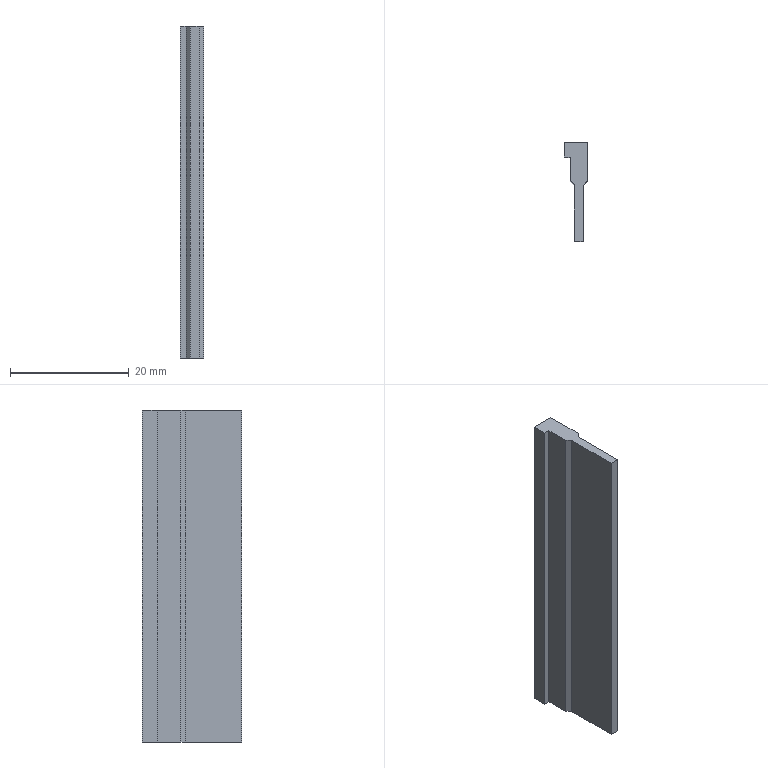Part | NX | features BREP 2 | 2 solids | 24 faces | box 3.95 x 16.702 x 56 mm | volume 4199 mm3 | plane 24
STEP:
#1=CARTESIAN_POINT('',(1.225,-8.351,-4.));
#2=VERTEX_POINT('',#1);
#3=CARTESIAN_POINT('',(1.225,-8.351,52.));
#4=VERTEX_POINT('',#3);
#5=CARTESIAN_POINT('',(1.225,-8.351,0.));
#6=DIRECTION('',(0.,0.,1.));
#7=VECTOR('',#6,1000.);
#8=LINE('',#5,#7);
#9=EDGE_CURVE('',#2,#4,#8,.T.);
#10=ORIENTED_EDGE('',*,*,#9,.F.);
#11=CARTESIAN_POINT('',(1.225,1.11,-4.));
#12=VERTEX_POINT('',#11);
#13=CARTESIAN_POINT('',(1.225,-22.649,-4.));
#14=DIRECTION('',(0.,1.,0.));
#15=VECTOR('',#14,1000.);
#16=LINE('',#13,#15);
#17=EDGE_CURVE('',#2,#12,#16,.T.);
#18=ORIENTED_EDGE('',*,*,#17,.T.);
#19=CARTESIAN_POINT('',(1.225,1.11,52.));
#20=VERTEX_POINT('',#19);
#21=CARTESIAN_POINT('',(1.225,1.11,0.));
#22=DIRECTION('',(0.,0.,1.));
#23=VECTOR('',#22,1000.);
#24=LINE('',#21,#23);
#25=EDGE_CURVE('',#12,#20,#24,.T.);
#26=ORIENTED_EDGE('',*,*,#25,.T.);
#27=CARTESIAN_POINT('',(1.225,-22.649,52.));
#28=DIRECTION('',(0.,1.,0.));
#29=VECTOR('',#28,1000.);
#30=LINE('',#27,#29);
#31=EDGE_CURVE('',#4,#20,#30,.T.);
#32=ORIENTED_EDGE('',*,*,#31,.F.);
#33=EDGE_LOOP('',(#10,#18,#26,#32));
#34=FACE_BOUND('',#33,.T.);
#35=CARTESIAN_POINT('',(1.225,-5.351,0.));
#36=DIRECTION('',(-1.,0.,0.));
#37=DIRECTION('',(0.,1.,0.));
#38=AXIS2_PLACEMENT_3D('',#35,#36,#37);
#39=PLANE('',#38);
#40=ADVANCED_FACE('',(#34),#39,.F.);
#41=ORIENTED_EDGE('',*,*,#9,.T.);
#42=CARTESIAN_POINT('',(-0.275,-8.351,52.));
#43=VERTEX_POINT('',#42);
#44=CARTESIAN_POINT('',(0.683,-8.351,52.));
#45=DIRECTION('',(1.,0.,0.));
#46=VECTOR('',#45,1000.);
#47=LINE('',#44,#46);
#48=EDGE_CURVE('',#43,#4,#47,.T.);
#49=ORIENTED_EDGE('',*,*,#48,.F.);
#50=CARTESIAN_POINT('',(-0.275,-8.351,-4.));
#51=VERTEX_POINT('',#50);
#52=CARTESIAN_POINT('',(-0.275,-8.351,0.));
#53=DIRECTION('',(0.,0.,1.));
#54=VECTOR('',#53,1000.);
#55=LINE('',#52,#54);
#56=EDGE_CURVE('',#51,#43,#55,.T.);
#57=ORIENTED_EDGE('',*,*,#56,.F.);
#58=CARTESIAN_POINT('',(0.683,-8.351,-4.));
#59=DIRECTION('',(1.,0.,0.));
#60=VECTOR('',#59,1000.);
#61=LINE('',#58,#60);
#62=EDGE_CURVE('',#51,#2,#61,.T.);
#63=ORIENTED_EDGE('',*,*,#62,.T.);
#64=EDGE_LOOP('',(#41,#49,#57,#63));
#65=FACE_BOUND('',#64,.T.);
#66=CARTESIAN_POINT('',(0.683,-8.351,0.));
#67=DIRECTION('',(0.,-1.,0.));
#68=DIRECTION('',(-1.,0.,0.));
#69=AXIS2_PLACEMENT_3D('',#66,#67,#68);
#70=PLANE('',#69);
#71=ADVANCED_FACE('',(#65),#70,.T.);
#72=CARTESIAN_POINT('',(-0.275,1.16,-4.));
#73=VERTEX_POINT('',#72);
#74=CARTESIAN_POINT('',(-0.275,1.16,52.));
#75=VERTEX_POINT('',#74);
#76=CARTESIAN_POINT('',(-0.275,1.16,0.));
#77=DIRECTION('',(0.,0.,1.));
#78=VECTOR('',#77,1000.);
#79=LINE('',#76,#78);
#80=EDGE_CURVE('',#73,#75,#79,.T.);
#81=ORIENTED_EDGE('',*,*,#80,.F.);
#82=CARTESIAN_POINT('',(-0.275,-22.649,-4.));
#83=DIRECTION('',(0.,-1.,0.));
#84=VECTOR('',#83,1000.);
#85=LINE('',#82,#84);
#86=EDGE_CURVE('',#73,#51,#85,.T.);
#87=ORIENTED_EDGE('',*,*,#86,.T.);
#88=ORIENTED_EDGE('',*,*,#56,.T.);
#89=CARTESIAN_POINT('',(-0.275,-22.649,52.));
#90=DIRECTION('',(0.,-1.,0.));
#91=VECTOR('',#90,1000.);
#92=LINE('',#89,#91);
#93=EDGE_CURVE('',#75,#43,#92,.T.);
#94=ORIENTED_EDGE('',*,*,#93,.F.);
#95=EDGE_LOOP('',(#81,#87,#88,#94));
#96=FACE_BOUND('',#95,.T.);
#97=CARTESIAN_POINT('',(-0.275,-4.148,0.));
#98=DIRECTION('',(1.,0.,0.));
#99=DIRECTION('',(0.,-1.,0.));
#100=AXIS2_PLACEMENT_3D('',#97,#98,#99);
#101=PLANE('',#100);
#102=ADVANCED_FACE('',(#96),#101,.F.);
#103=ORIENTED_EDGE('',*,*,#80,.T.);
#104=CARTESIAN_POINT('',(-0.975,1.86,52.));
#105=VERTEX_POINT('',#104);
#106=CARTESIAN_POINT('',(-0.275,1.16,52.));
#107=DIRECTION('',(0.7071,-0.7071,0.));
#108=VECTOR('',#107,1000.);
#109=LINE('',#106,#108);
#110=EDGE_CURVE('',#105,#75,#109,.T.);
#111=ORIENTED_EDGE('',*,*,#110,.F.);
#112=CARTESIAN_POINT('',(-0.975,1.86,-4.));
#113=VERTEX_POINT('',#112);
#114=CARTESIAN_POINT('',(-0.975,1.86,0.));
#115=DIRECTION('',(0.,0.,1.));
#116=VECTOR('',#115,1000.);
#117=LINE('',#114,#116);
#118=EDGE_CURVE('',#113,#105,#117,.T.);
#119=ORIENTED_EDGE('',*,*,#118,.F.);
#120=CARTESIAN_POINT('',(-0.275,1.16,-4.));
#121=DIRECTION('',(0.7071,-0.7071,0.));
#122=VECTOR('',#121,1000.);
#123=LINE('',#120,#122);
#124=EDGE_CURVE('',#113,#73,#123,.T.);
#125=ORIENTED_EDGE('',*,*,#124,.T.);
#126=EDGE_LOOP('',(#103,#111,#119,#125));
#127=FACE_BOUND('',#126,.T.);
#128=CARTESIAN_POINT('',(-0.275,1.16,0.));
#129=DIRECTION('',(0.7071,0.7071,0.));
#130=DIRECTION('',(0.7071,-0.7071,0.));
#131=AXIS2_PLACEMENT_3D('',#128,#129,#130);
#132=PLANE('',#131);
#133=ADVANCED_FACE('',(#127),#132,.F.);
#134=ORIENTED_EDGE('',*,*,#118,.T.);
#135=CARTESIAN_POINT('',(-0.975,5.852,52.));
#136=VERTEX_POINT('',#135);
#137=CARTESIAN_POINT('',(-0.975,-22.649,52.));
#138=DIRECTION('',(0.,-1.,0.));
#139=VECTOR('',#138,1000.);
#140=LINE('',#137,#139);
#141=EDGE_CURVE('',#136,#105,#140,.T.);
#142=ORIENTED_EDGE('',*,*,#141,.F.);
#143=CARTESIAN_POINT('',(-0.975,5.852,-4.));
#144=VERTEX_POINT('',#143);
#145=CARTESIAN_POINT('',(-0.975,5.852,0.));
#146=DIRECTION('',(0.,0.,1.));
#147=VECTOR('',#146,1000.);
#148=LINE('',#145,#147);
#149=EDGE_CURVE('',#144,#136,#148,.T.);
#150=ORIENTED_EDGE('',*,*,#149,.F.);
#151=CARTESIAN_POINT('',(-0.975,-22.649,-4.));
#152=DIRECTION('',(0.,-1.,0.));
#153=VECTOR('',#152,1000.);
#154=LINE('',#151,#153);
#155=EDGE_CURVE('',#144,#113,#154,.T.);
#156=ORIENTED_EDGE('',*,*,#155,.T.);
#157=EDGE_LOOP('',(#134,#142,#150,#156));
#158=FACE_BOUND('',#157,.T.);
#159=CARTESIAN_POINT('',(-0.975,1.86,0.));
#160=DIRECTION('',(1.,0.,0.));
#161=DIRECTION('',(0.,-1.,0.));
#162=AXIS2_PLACEMENT_3D('',#159,#160,#161);
#163=PLANE('',#162);
#164=ADVANCED_FACE('',(#158),#163,.F.);
#165=ORIENTED_EDGE('',*,*,#149,.T.);
#166=CARTESIAN_POINT('',(-1.975,5.852,52.));
#167=VERTEX_POINT('',#166);
#168=CARTESIAN_POINT('',(0.683,5.852,52.));
#169=DIRECTION('',(1.,0.,0.));
#170=VECTOR('',#169,1000.);
#171=LINE('',#168,#170);
#172=EDGE_CURVE('',#167,#136,#171,.T.);
#173=ORIENTED_EDGE('',*,*,#172,.F.);
#174=CARTESIAN_POINT('',(-1.975,5.852,-4.));
#175=VERTEX_POINT('',#174);
#176=CARTESIAN_POINT('',(-1.975,5.852,0.));
#177=DIRECTION('',(0.,0.,1.));
#178=VECTOR('',#177,1000.);
#179=LINE('',#176,#178);
#180=EDGE_CURVE('',#175,#167,#179,.T.);
#181=ORIENTED_EDGE('',*,*,#180,.F.);
#182=CARTESIAN_POINT('',(0.683,5.852,-4.));
#183=DIRECTION('',(1.,0.,0.));
#184=VECTOR('',#183,1000.);
#185=LINE('',#182,#184);
#186=EDGE_CURVE('',#175,#144,#185,.T.);
#187=ORIENTED_EDGE('',*,*,#186,.T.);
#188=EDGE_LOOP('',(#165,#173,#181,#187));
#189=FACE_BOUND('',#188,.T.);
#190=CARTESIAN_POINT('',(-0.975,5.852,0.));
#191=DIRECTION('',(0.,1.,0.));
#192=DIRECTION('',(1.,0.,0.));
#193=AXIS2_PLACEMENT_3D('',#190,#191,#192);
#194=PLANE('',#193);
#195=ADVANCED_FACE('',(#189),#194,.F.);
#196=ORIENTED_EDGE('',*,*,#180,.T.);
#197=CARTESIAN_POINT('',(-1.975,8.351,52.));
#198=VERTEX_POINT('',#197);
#199=CARTESIAN_POINT('',(-1.975,-22.649,52.));
#200=DIRECTION('',(0.,-1.,0.));
#201=VECTOR('',#200,1000.);
#202=LINE('',#199,#201);
#203=EDGE_CURVE('',#198,#167,#202,.T.);
#204=ORIENTED_EDGE('',*,*,#203,.F.);
#205=CARTESIAN_POINT('',(-1.975,8.351,-4.));
#206=VERTEX_POINT('',#205);
#207=CARTESIAN_POINT('',(-1.975,8.351,0.));
#208=DIRECTION('',(0.,0.,1.));
#209=VECTOR('',#208,1000.);
#210=LINE('',#207,#209);
#211=EDGE_CURVE('',#206,#198,#210,.T.);
#212=ORIENTED_EDGE('',*,*,#211,.F.);
#213=CARTESIAN_POINT('',(-1.975,-22.649,-4.));
#214=DIRECTION('',(0.,-1.,0.));
#215=VECTOR('',#214,1000.);
#216=LINE('',#213,#215);
#217=EDGE_CURVE('',#206,#175,#216,.T.);
#218=ORIENTED_EDGE('',*,*,#217,.T.);
#219=EDGE_LOOP('',(#196,#204,#212,#218));
#220=FACE_BOUND('',#219,.T.);
#221=CARTESIAN_POINT('',(-1.975,-22.649,0.));
#222=DIRECTION('',(1.,0.,0.));
#223=DIRECTION('',(0.,-1.,0.));
#224=AXIS2_PLACEMENT_3D('',#221,#222,#223);
#225=PLANE('',#224);
#226=ADVANCED_FACE('',(#220),#225,.F.);
#227=ORIENTED_EDGE('',*,*,#211,.T.);
#228=CARTESIAN_POINT('',(1.975,8.351,52.));
#229=VERTEX_POINT('',#228);
#230=CARTESIAN_POINT('',(0.683,8.351,52.));
#231=DIRECTION('',(-1.,0.,0.));
#232=VECTOR('',#231,1000.);
#233=LINE('',#230,#232);
#234=EDGE_CURVE('',#229,#198,#233,.T.);
#235=ORIENTED_EDGE('',*,*,#234,.F.);
#236=CARTESIAN_POINT('',(1.975,8.351,-4.));
#237=VERTEX_POINT('',#236);
#238=CARTESIAN_POINT('',(1.975,8.351,0.));
#239=DIRECTION('',(0.,0.,1.));
#240=VECTOR('',#239,1000.);
#241=LINE('',#238,#240);
#242=EDGE_CURVE('',#237,#229,#241,.T.);
#243=ORIENTED_EDGE('',*,*,#242,.F.);
#244=CARTESIAN_POINT('',(0.683,8.351,-4.));
#245=DIRECTION('',(-1.,0.,0.));
#246=VECTOR('',#245,1000.);
#247=LINE('',#244,#246);
#248=EDGE_CURVE('',#237,#206,#247,.T.);
#249=ORIENTED_EDGE('',*,*,#248,.T.);
#250=EDGE_LOOP('',(#227,#235,#243,#249));
#251=FACE_BOUND('',#250,.T.);
#252=CARTESIAN_POINT('',(-21.567,8.351,0.));
#253=DIRECTION('',(0.,-1.,0.));
#254=DIRECTION('',(-1.,0.,0.));
#255=AXIS2_PLACEMENT_3D('',#252,#253,#254);
#256=PLANE('',#255);
#257=ADVANCED_FACE('',(#251),#256,.F.);
#258=ORIENTED_EDGE('',*,*,#242,.T.);
#259=CARTESIAN_POINT('',(1.975,1.86,52.));
#260=VERTEX_POINT('',#259);
#261=CARTESIAN_POINT('',(1.975,-22.649,52.));
#262=DIRECTION('',(0.,1.,0.));
#263=VECTOR('',#262,1000.);
#264=LINE('',#261,#263);
#265=EDGE_CURVE('',#260,#229,#264,.T.);
#266=ORIENTED_EDGE('',*,*,#265,.F.);
#267=CARTESIAN_POINT('',(1.975,1.86,-4.));
#268=VERTEX_POINT('',#267);
#269=CARTESIAN_POINT('',(1.975,1.86,0.));
#270=DIRECTION('',(0.,0.,1.));
#271=VECTOR('',#270,1000.);
#272=LINE('',#269,#271);
#273=EDGE_CURVE('',#268,#260,#272,.T.);
#274=ORIENTED_EDGE('',*,*,#273,.F.);
#275=CARTESIAN_POINT('',(1.975,-22.649,-4.));
#276=DIRECTION('',(0.,1.,0.));
#277=VECTOR('',#276,1000.);
#278=LINE('',#275,#277);
#279=EDGE_CURVE('',#268,#237,#278,.T.);
#280=ORIENTED_EDGE('',*,*,#279,.T.);
#281=EDGE_LOOP('',(#258,#266,#274,#280));
#282=FACE_BOUND('',#281,.T.);
#283=CARTESIAN_POINT('',(1.975,5.852,0.));
#284=DIRECTION('',(-1.,0.,0.));
#285=DIRECTION('',(0.,1.,0.));
#286=AXIS2_PLACEMENT_3D('',#283,#284,#285);
#287=PLANE('',#286);
#288=ADVANCED_FACE('',(#282),#287,.F.);
#289=CARTESIAN_POINT('',(1.975,1.86,-4.));
#290=DIRECTION('',(0.7071,0.7071,0.));
#291=VECTOR('',#290,1000.);
#292=LINE('',#289,#291);
#293=EDGE_CURVE('',#12,#268,#292,.T.);
#294=ORIENTED_EDGE('',*,*,#293,.T.);
#295=ORIENTED_EDGE('',*,*,#273,.T.);
#296=CARTESIAN_POINT('',(1.975,1.86,52.));
#297=DIRECTION('',(0.7071,0.7071,0.));
#298=VECTOR('',#297,1000.);
#299=LINE('',#296,#298);
#300=EDGE_CURVE('',#20,#260,#299,.T.);
#301=ORIENTED_EDGE('',*,*,#300,.F.);
#302=ORIENTED_EDGE('',*,*,#25,.F.);
#303=EDGE_LOOP('',(#294,#295,#301,#302));
#304=FACE_BOUND('',#303,.T.);
#305=CARTESIAN_POINT('',(1.975,1.86,0.));
#306=DIRECTION('',(-0.7071,0.7071,0.));
#307=DIRECTION('',(0.7071,0.7071,0.));
#308=AXIS2_PLACEMENT_3D('',#305,#306,#307);
#309=PLANE('',#308);
#310=ADVANCED_FACE('',(#304),#309,.F.);
#311=ORIENTED_EDGE('',*,*,#265,.T.);
#312=ORIENTED_EDGE('',*,*,#234,.T.);
#313=ORIENTED_EDGE('',*,*,#203,.T.);
#314=ORIENTED_EDGE('',*,*,#172,.T.);
#315=ORIENTED_EDGE('',*,*,#141,.T.);
#316=ORIENTED_EDGE('',*,*,#110,.T.);
#317=ORIENTED_EDGE('',*,*,#93,.T.);
#318=ORIENTED_EDGE('',*,*,#48,.T.);
#319=ORIENTED_EDGE('',*,*,#31,.T.);
#320=ORIENTED_EDGE('',*,*,#300,.T.);
#321=EDGE_LOOP('',(#311,#312,#313,#314,#315,#316,#317,#318,#319,#320));
#322=FACE_BOUND('',#321,.T.);
#323=CARTESIAN_POINT('',(0.683,-22.649,52.));
#324=DIRECTION('',(0.,0.,1.));
#325=DIRECTION('',(-1.,0.,0.));
#326=AXIS2_PLACEMENT_3D('',#323,#324,#325);
#327=PLANE('',#326);
#328=ADVANCED_FACE('',(#322),#327,.T.);
#329=ORIENTED_EDGE('',*,*,#279,.F.);
#330=ORIENTED_EDGE('',*,*,#293,.F.);
#331=ORIENTED_EDGE('',*,*,#17,.F.);
#332=ORIENTED_EDGE('',*,*,#62,.F.);
#333=ORIENTED_EDGE('',*,*,#86,.F.);
#334=ORIENTED_EDGE('',*,*,#124,.F.);
#335=ORIENTED_EDGE('',*,*,#155,.F.);
#336=ORIENTED_EDGE('',*,*,#186,.F.);
#337=ORIENTED_EDGE('',*,*,#217,.F.);
#338=ORIENTED_EDGE('',*,*,#248,.F.);
#339=EDGE_LOOP('',(#329,#330,#331,#332,#333,#334,#335,#336,#337,#338));
#340=FACE_BOUND('',#339,.T.);
#341=CARTESIAN_POINT('',(0.683,-22.649,-4.));
#342=DIRECTION('',(0.,0.,1.));
#343=DIRECTION('',(-1.,0.,0.));
#344=AXIS2_PLACEMENT_3D('',#341,#342,#343);
#345=PLANE('',#344);
#346=ADVANCED_FACE('',(#340),#345,.F.);
#347=CLOSED_SHELL('',(#40,#71,#102,#133,#164,#195,#226,#257,#288,#310,#328,#346));
#348=MANIFOLD_SOLID_BREP('',#347);
#349=CARTESIAN_POINT('',(1.225,-8.351,-4.));
#350=VERTEX_POINT('',#349);
#351=CARTESIAN_POINT('',(1.225,-8.351,52.));
#352=VERTEX_POINT('',#351);
#353=CARTESIAN_POINT('',(1.225,-8.351,0.));
#354=DIRECTION('',(0.,0.,1.));
#355=VECTOR('',#354,1000.);
#356=LINE('',#353,#355);
#357=EDGE_CURVE('',#350,#352,#356,.T.);
#358=ORIENTED_EDGE('',*,*,#357,.F.);
#359=CARTESIAN_POINT('',(1.225,1.11,-4.));
#360=VERTEX_POINT('',#359);
#361=CARTESIAN_POINT('',(1.225,-22.649,-4.));
#362=DIRECTION('',(0.,1.,0.));
#363=VECTOR('',#362,1000.);
#364=LINE('',#361,#363);
#365=EDGE_CURVE('',#350,#360,#364,.T.);
#366=ORIENTED_EDGE('',*,*,#365,.T.);
#367=CARTESIAN_POINT('',(1.225,1.11,52.));
#368=VERTEX_POINT('',#367);
#369=CARTESIAN_POINT('',(1.225,1.11,0.));
#370=DIRECTION('',(0.,0.,1.));
#371=VECTOR('',#370,1000.);
#372=LINE('',#369,#371);
#373=EDGE_CURVE('',#360,#368,#372,.T.);
#374=ORIENTED_EDGE('',*,*,#373,.T.);
#375=CARTESIAN_POINT('',(1.225,-22.649,52.));
#376=DIRECTION('',(0.,1.,0.));
#377=VECTOR('',#376,1000.);
#378=LINE('',#375,#377);
#379=EDGE_CURVE('',#352,#368,#378,.T.);
#380=ORIENTED_EDGE('',*,*,#379,.F.);
#381=EDGE_LOOP('',(#358,#366,#374,#380));
#382=FACE_BOUND('',#381,.T.);
#383=CARTESIAN_POINT('',(1.225,-5.351,0.));
#384=DIRECTION('',(-1.,0.,0.));
#385=DIRECTION('',(0.,1.,0.));
#386=AXIS2_PLACEMENT_3D('',#383,#384,#385);
#387=PLANE('',#386);
#388=ADVANCED_FACE('',(#382),#387,.F.);
#389=ORIENTED_EDGE('',*,*,#357,.T.);
#390=CARTESIAN_POINT('',(-0.275,-8.351,52.));
#391=VERTEX_POINT('',#390);
#392=CARTESIAN_POINT('',(0.683,-8.351,52.));
#393=DIRECTION('',(1.,0.,0.));
#394=VECTOR('',#393,1000.);
#395=LINE('',#392,#394);
#396=EDGE_CURVE('',#391,#352,#395,.T.);
#397=ORIENTED_EDGE('',*,*,#396,.F.);
#398=CARTESIAN_POINT('',(-0.275,-8.351,-4.));
#399=VERTEX_POINT('',#398);
#400=CARTESIAN_POINT('',(-0.275,-8.351,0.));
#401=DIRECTION('',(0.,0.,1.));
#402=VECTOR('',#401,1000.);
#403=LINE('',#400,#402);
#404=EDGE_CURVE('',#399,#391,#403,.T.);
#405=ORIENTED_EDGE('',*,*,#404,.F.);
#406=CARTESIAN_POINT('',(0.683,-8.351,-4.));
#407=DIRECTION('',(1.,0.,0.));
#408=VECTOR('',#407,1000.);
#409=LINE('',#406,#408);
#410=EDGE_CURVE('',#399,#350,#409,.T.);
#411=ORIENTED_EDGE('',*,*,#410,.T.);
#412=EDGE_LOOP('',(#389,#397,#405,#411));
#413=FACE_BOUND('',#412,.T.);
#414=CARTESIAN_POINT('',(0.683,-8.351,0.));
#415=DIRECTION('',(0.,-1.,0.));
#416=DIRECTION('',(-1.,0.,0.));
#417=AXIS2_PLACEMENT_3D('',#414,#415,#416);
#418=PLANE('',#417);
#419=ADVANCED_FACE('',(#413),#418,.T.);
#420=CARTESIAN_POINT('',(-0.275,1.16,-4.));
#421=VERTEX_POINT('',#420);
#422=CARTESIAN_POINT('',(-0.275,1.16,52.));
#423=VERTEX_POINT('',#422);
#424=CARTESIAN_POINT('',(-0.275,1.16,0.));
#425=DIRECTION('',(0.,0.,1.));
#426=VECTOR('',#425,1000.);
#427=LINE('',#424,#426);
#428=EDGE_CURVE('',#421,#423,#427,.T.);
#429=ORIENTED_EDGE('',*,*,#428,.F.);
#430=CARTESIAN_POINT('',(-0.275,-22.649,-4.));
#431=DIRECTION('',(0.,-1.,0.));
#432=VECTOR('',#431,1000.);
#433=LINE('',#430,#432);
#434=EDGE_CURVE('',#421,#399,#433,.T.);
#435=ORIENTED_EDGE('',*,*,#434,.T.);
#436=ORIENTED_EDGE('',*,*,#404,.T.);
#437=CARTESIAN_POINT('',(-0.275,-22.649,52.));
#438=DIRECTION('',(0.,-1.,0.));
#439=VECTOR('',#438,1000.);
#440=LINE('',#437,#439);
#441=EDGE_CURVE('',#423,#391,#440,.T.);
#442=ORIENTED_EDGE('',*,*,#441,.F.);
#443=EDGE_LOOP('',(#429,#435,#436,#442));
#444=FACE_BOUND('',#443,.T.);
#445=CARTESIAN_POINT('',(-0.275,-4.148,0.));
#446=DIRECTION('',(1.,0.,0.));
#447=DIRECTION('',(0.,-1.,0.));
#448=AXIS2_PLACEMENT_3D('',#445,#446,#447);
#449=PLANE('',#448);
#450=ADVANCED_FACE('',(#444),#449,.F.);
#451=ORIENTED_EDGE('',*,*,#428,.T.);
#452=CARTESIAN_POINT('',(-0.975,1.86,52.));
#453=VERTEX_POINT('',#452);
#454=CARTESIAN_POINT('',(-0.275,1.16,52.));
#455=DIRECTION('',(0.7071,-0.7071,0.));
#456=VECTOR('',#455,1000.);
#457=LINE('',#454,#456);
#458=EDGE_CURVE('',#453,#423,#457,.T.);
#459=ORIENTED_EDGE('',*,*,#458,.F.);
#460=CARTESIAN_POINT('',(-0.975,1.86,-4.));
#461=VERTEX_POINT('',#460);
#462=CARTESIAN_POINT('',(-0.975,1.86,0.));
#463=DIRECTION('',(0.,0.,1.));
#464=VECTOR('',#463,1000.);
#465=LINE('',#462,#464);
#466=EDGE_CURVE('',#461,#453,#465,.T.);
#467=ORIENTED_EDGE('',*,*,#466,.F.);
#468=CARTESIAN_POINT('',(-0.275,1.16,-4.));
#469=DIRECTION('',(0.7071,-0.7071,0.));
#470=VECTOR('',#469,1000.);
#471=LINE('',#468,#470);
#472=EDGE_CURVE('',#461,#421,#471,.T.);
#473=ORIENTED_EDGE('',*,*,#472,.T.);
#474=EDGE_LOOP('',(#451,#459,#467,#473));
#475=FACE_BOUND('',#474,.T.);
#476=CARTESIAN_POINT('',(-0.275,1.16,0.));
#477=DIRECTION('',(0.7071,0.7071,0.));
#478=DIRECTION('',(0.7071,-0.7071,0.));
#479=AXIS2_PLACEMENT_3D('',#476,#477,#478);
#480=PLANE('',#479);
#481=ADVANCED_FACE('',(#475),#480,.F.);
#482=ORIENTED_EDGE('',*,*,#466,.T.);
#483=CARTESIAN_POINT('',(-0.975,5.852,52.));
#484=VERTEX_POINT('',#483);
#485=CARTESIAN_POINT('',(-0.975,-22.649,52.));
#486=DIRECTION('',(0.,-1.,0.));
#487=VECTOR('',#486,1000.);
#488=LINE('',#485,#487);
#489=EDGE_CURVE('',#484,#453,#488,.T.);
#490=ORIENTED_EDGE('',*,*,#489,.F.);
#491=CARTESIAN_POINT('',(-0.975,5.852,-4.));
#492=VERTEX_POINT('',#491);
#493=CARTESIAN_POINT('',(-0.975,5.852,0.));
#494=DIRECTION('',(0.,0.,1.));
#495=VECTOR('',#494,1000.);
#496=LINE('',#493,#495);
#497=EDGE_CURVE('',#492,#484,#496,.T.);
#498=ORIENTED_EDGE('',*,*,#497,.F.);
#499=CARTESIAN_POINT('',(-0.975,-22.649,-4.));
#500=DIRECTION('',(0.,-1.,0.));
#501=VECTOR('',#500,1000.);
#502=LINE('',#499,#501);
#503=EDGE_CURVE('',#492,#461,#502,.T.);
#504=ORIENTED_EDGE('',*,*,#503,.T.);
#505=EDGE_LOOP('',(#482,#490,#498,#504));
#506=FACE_BOUND('',#505,.T.);
#507=CARTESIAN_POINT('',(-0.975,1.86,0.));
#508=DIRECTION('',(1.,0.,0.));
#509=DIRECTION('',(0.,-1.,0.));
#510=AXIS2_PLACEMENT_3D('',#507,#508,#509);
#511=PLANE('',#510);
#512=ADVANCED_FACE('',(#506),#511,.F.);
#513=ORIENTED_EDGE('',*,*,#497,.T.);
#514=CARTESIAN_POINT('',(-1.975,5.852,52.));
#515=VERTEX_POINT('',#514);
#516=CARTESIAN_POINT('',(0.683,5.852,52.));
#517=DIRECTION('',(1.,0.,0.));
#518=VECTOR('',#517,1000.);
#519=LINE('',#516,#518);
#520=EDGE_CURVE('',#515,#484,#519,.T.);
#521=ORIENTED_EDGE('',*,*,#520,.F.);
#522=CARTESIAN_POINT('',(-1.975,5.852,-4.));
#523=VERTEX_POINT('',#522);
#524=CARTESIAN_POINT('',(-1.975,5.852,0.));
#525=DIRECTION('',(0.,0.,1.));
#526=VECTOR('',#525,1000.);
#527=LINE('',#524,#526);
#528=EDGE_CURVE('',#523,#515,#527,.T.);
#529=ORIENTED_EDGE('',*,*,#528,.F.);
#530=CARTESIAN_POINT('',(0.683,5.852,-4.));
#531=DIRECTION('',(1.,0.,0.));
#532=VECTOR('',#531,1000.);
#533=LINE('',#530,#532);
#534=EDGE_CURVE('',#523,#492,#533,.T.);
#535=ORIENTED_EDGE('',*,*,#534,.T.);
#536=EDGE_LOOP('',(#513,#521,#529,#535));
#537=FACE_BOUND('',#536,.T.);
#538=CARTESIAN_POINT('',(-0.975,5.852,0.));
#539=DIRECTION('',(0.,1.,0.));
#540=DIRECTION('',(1.,0.,0.));
#541=AXIS2_PLACEMENT_3D('',#538,#539,#540);
#542=PLANE('',#541);
#543=ADVANCED_FACE('',(#537),#542,.F.);
#544=ORIENTED_EDGE('',*,*,#528,.T.);
#545=CARTESIAN_POINT('',(-1.975,8.351,52.));
#546=VERTEX_POINT('',#545);
#547=CARTESIAN_POINT('',(-1.975,-22.649,52.));
#548=DIRECTION('',(0.,-1.,0.));
#549=VECTOR('',#548,1000.);
#550=LINE('',#547,#549);
#551=EDGE_CURVE('',#546,#515,#550,.T.);
#552=ORIENTED_EDGE('',*,*,#551,.F.);
#553=CARTESIAN_POINT('',(-1.975,8.351,-4.));
#554=VERTEX_POINT('',#553);
#555=CARTESIAN_POINT('',(-1.975,8.351,0.));
#556=DIRECTION('',(0.,0.,1.));
#557=VECTOR('',#556,1000.);
#558=LINE('',#555,#557);
#559=EDGE_CURVE('',#554,#546,#558,.T.);
#560=ORIENTED_EDGE('',*,*,#559,.F.);
#561=CARTESIAN_POINT('',(-1.975,-22.649,-4.));
#562=DIRECTION('',(0.,-1.,0.));
#563=VECTOR('',#562,1000.);
#564=LINE('',#561,#563);
#565=EDGE_CURVE('',#554,#523,#564,.T.);
#566=ORIENTED_EDGE('',*,*,#565,.T.);
#567=EDGE_LOOP('',(#544,#552,#560,#566));
#568=FACE_BOUND('',#567,.T.);
#569=CARTESIAN_POINT('',(-1.975,-22.649,0.));
#570=DIRECTION('',(1.,0.,0.));
#571=DIRECTION('',(0.,-1.,0.));
#572=AXIS2_PLACEMENT_3D('',#569,#570,#571);
#573=PLANE('',#572);
#574=ADVANCED_FACE('',(#568),#573,.F.);
#575=ORIENTED_EDGE('',*,*,#559,.T.);
#576=CARTESIAN_POINT('',(1.975,8.351,52.));
#577=VERTEX_POINT('',#576);
#578=CARTESIAN_POINT('',(0.683,8.351,52.));
#579=DIRECTION('',(-1.,0.,0.));
#580=VECTOR('',#579,1000.);
#581=LINE('',#578,#580);
#582=EDGE_CURVE('',#577,#546,#581,.T.);
#583=ORIENTED_EDGE('',*,*,#582,.F.);
#584=CARTESIAN_POINT('',(1.975,8.351,-4.));
#585=VERTEX_POINT('',#584);
#586=CARTESIAN_POINT('',(1.975,8.351,0.));
#587=DIRECTION('',(0.,0.,1.));
#588=VECTOR('',#587,1000.);
#589=LINE('',#586,#588);
#590=EDGE_CURVE('',#585,#577,#589,.T.);
#591=ORIENTED_EDGE('',*,*,#590,.F.);
#592=CARTESIAN_POINT('',(0.683,8.351,-4.));
#593=DIRECTION('',(-1.,0.,0.));
#594=VECTOR('',#593,1000.);
#595=LINE('',#592,#594);
#596=EDGE_CURVE('',#585,#554,#595,.T.);
#597=ORIENTED_EDGE('',*,*,#596,.T.);
#598=EDGE_LOOP('',(#575,#583,#591,#597));
#599=FACE_BOUND('',#598,.T.);
#600=CARTESIAN_POINT('',(-21.567,8.351,0.));
#601=DIRECTION('',(0.,-1.,0.));
#602=DIRECTION('',(-1.,0.,0.));
#603=AXIS2_PLACEMENT_3D('',#600,#601,#602);
#604=PLANE('',#603);
#605=ADVANCED_FACE('',(#599),#604,.F.);
#606=ORIENTED_EDGE('',*,*,#590,.T.);
#607=CARTESIAN_POINT('',(1.975,1.86,52.));
#608=VERTEX_POINT('',#607);
#609=CARTESIAN_POINT('',(1.975,-22.649,52.));
#610=DIRECTION('',(0.,1.,0.));
#611=VECTOR('',#610,1000.);
#612=LINE('',#609,#611);
#613=EDGE_CURVE('',#608,#577,#612,.T.);
#614=ORIENTED_EDGE('',*,*,#613,.F.);
#615=CARTESIAN_POINT('',(1.975,1.86,-4.));
#616=VERTEX_POINT('',#615);
#617=CARTESIAN_POINT('',(1.975,1.86,0.));
#618=DIRECTION('',(0.,0.,1.));
#619=VECTOR('',#618,1000.);
#620=LINE('',#617,#619);
#621=EDGE_CURVE('',#616,#608,#620,.T.);
#622=ORIENTED_EDGE('',*,*,#621,.F.);
#623=CARTESIAN_POINT('',(1.975,-22.649,-4.));
#624=DIRECTION('',(0.,1.,0.));
#625=VECTOR('',#624,1000.);
#626=LINE('',#623,#625);
#627=EDGE_CURVE('',#616,#585,#626,.T.);
#628=ORIENTED_EDGE('',*,*,#627,.T.);
#629=EDGE_LOOP('',(#606,#614,#622,#628));
#630=FACE_BOUND('',#629,.T.);
#631=CARTESIAN_POINT('',(1.975,5.852,0.));
#632=DIRECTION('',(-1.,0.,0.));
#633=DIRECTION('',(0.,1.,0.));
#634=AXIS2_PLACEMENT_3D('',#631,#632,#633);
#635=PLANE('',#634);
#636=ADVANCED_FACE('',(#630),#635,.F.);
#637=CARTESIAN_POINT('',(1.975,1.86,-4.));
#638=DIRECTION('',(0.7071,0.7071,0.));
#639=VECTOR('',#638,1000.);
#640=LINE('',#637,#639);
#641=EDGE_CURVE('',#360,#616,#640,.T.);
#642=ORIENTED_EDGE('',*,*,#641,.T.);
#643=ORIENTED_EDGE('',*,*,#621,.T.);
#644=CARTESIAN_POINT('',(1.975,1.86,52.));
#645=DIRECTION('',(0.7071,0.7071,0.));
#646=VECTOR('',#645,1000.);
#647=LINE('',#644,#646);
#648=EDGE_CURVE('',#368,#608,#647,.T.);
#649=ORIENTED_EDGE('',*,*,#648,.F.);
#650=ORIENTED_EDGE('',*,*,#373,.F.);
#651=EDGE_LOOP('',(#642,#643,#649,#650));
#652=FACE_BOUND('',#651,.T.);
#653=CARTESIAN_POINT('',(1.975,1.86,0.));
#654=DIRECTION('',(-0.7071,0.7071,0.));
#655=DIRECTION('',(0.7071,0.7071,0.));
#656=AXIS2_PLACEMENT_3D('',#653,#654,#655);
#657=PLANE('',#656);
#658=ADVANCED_FACE('',(#652),#657,.F.);
#659=ORIENTED_EDGE('',*,*,#613,.T.);
#660=ORIENTED_EDGE('',*,*,#582,.T.);
#661=ORIENTED_EDGE('',*,*,#551,.T.);
#662=ORIENTED_EDGE('',*,*,#520,.T.);
#663=ORIENTED_EDGE('',*,*,#489,.T.);
#664=ORIENTED_EDGE('',*,*,#458,.T.);
#665=ORIENTED_EDGE('',*,*,#441,.T.);
#666=ORIENTED_EDGE('',*,*,#396,.T.);
#667=ORIENTED_EDGE('',*,*,#379,.T.);
#668=ORIENTED_EDGE('',*,*,#648,.T.);
#669=EDGE_LOOP('',(#659,#660,#661,#662,#663,#664,#665,#666,#667,#668));
#670=FACE_BOUND('',#669,.T.);
#671=CARTESIAN_POINT('',(0.683,-22.649,52.));
#672=DIRECTION('',(0.,0.,1.));
#673=DIRECTION('',(-1.,0.,0.));
#674=AXIS2_PLACEMENT_3D('',#671,#672,#673);
#675=PLANE('',#674);
#676=ADVANCED_FACE('',(#670),#675,.T.);
#677=ORIENTED_EDGE('',*,*,#627,.F.);
#678=ORIENTED_EDGE('',*,*,#641,.F.);
#679=ORIENTED_EDGE('',*,*,#365,.F.);
#680=ORIENTED_EDGE('',*,*,#410,.F.);
#681=ORIENTED_EDGE('',*,*,#434,.F.);
#682=ORIENTED_EDGE('',*,*,#472,.F.);
#683=ORIENTED_EDGE('',*,*,#503,.F.);
#684=ORIENTED_EDGE('',*,*,#534,.F.);
#685=ORIENTED_EDGE('',*,*,#565,.F.);
#686=ORIENTED_EDGE('',*,*,#596,.F.);
#687=EDGE_LOOP('',(#677,#678,#679,#680,#681,#682,#683,#684,#685,#686));
#688=FACE_BOUND('',#687,.T.);
#689=CARTESIAN_POINT('',(0.683,-22.649,-4.));
#690=DIRECTION('',(0.,0.,1.));
#691=DIRECTION('',(-1.,0.,0.));
#692=AXIS2_PLACEMENT_3D('',#689,#690,#691);
#693=PLANE('',#692);
#694=ADVANCED_FACE('',(#688),#693,.F.);
#695=CLOSED_SHELL('',(#388,#419,#450,#481,#512,#543,#574,#605,#636,#658,#676,#694));
#696=MANIFOLD_SOLID_BREP('',#695);
#697=(LENGTH_UNIT()NAMED_UNIT(*)SI_UNIT(.MILLI.,.METRE.));
#698=UNCERTAINTY_MEASURE_WITH_UNIT(LENGTH_MEASURE(0.00001),#697,'','');
#699=(NAMED_UNIT(*)PLANE_ANGLE_UNIT()SI_UNIT($,.RADIAN.));
#700=(NAMED_UNIT(*)SI_UNIT($,.STERADIAN.)SOLID_ANGLE_UNIT());
#701=(GEOMETRIC_REPRESENTATION_CONTEXT(3)GLOBAL_UNCERTAINTY_ASSIGNED_CONTEXT((#698))GLOBAL_UNIT_ASSIGNED_CONTEXT((#697,#699,#700))REPRESENTATION_CONTEXT('',''));
#702=ADVANCED_BREP_SHAPE_REPRESENTATION('',(#348,#696),#701);